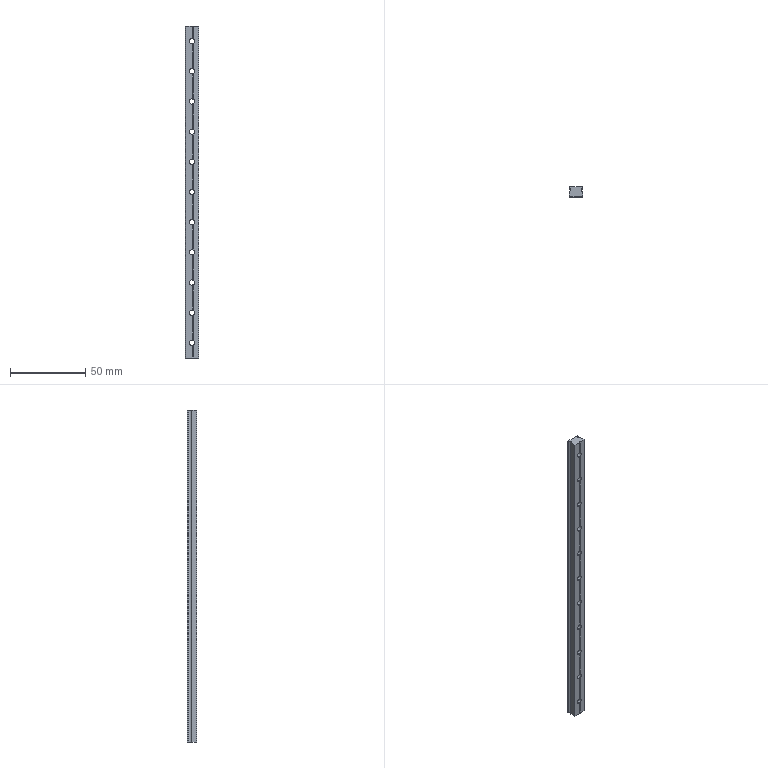Part | STEP file | Copy 1^MGN9C2R220Z0CM (11-hole centred E=10+10) | 1 solid | 83 faces | box 9 x 6.5 x 220 mm | volume 10729 mm3 | cylinder 59 | plane 24 | commonest cylinder face diameters 3.5 x22 6 x22 0.6 x12 2 x3